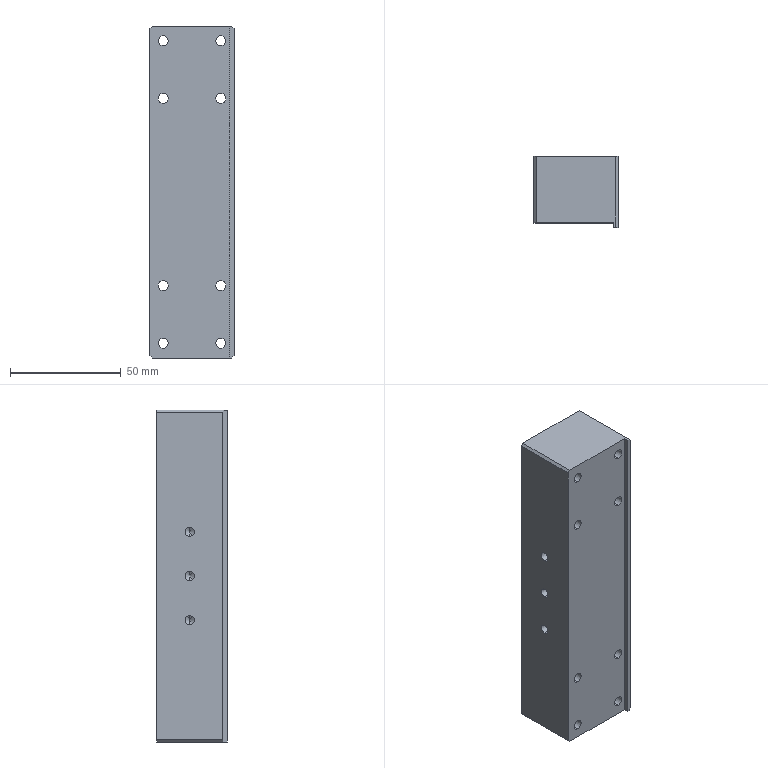Part | SolidWorks | features HoleWzd 4, Chamfer 1, Extrusion 1 | 1 solid | 92 faces | box 38 x 32 x 150 mm | volume 164701 mm3 | cylinder 52 | cone 20 | plane 20 | commonest cylinder face diameters 4.2 x18 4.5 x16 8 x16 5 x2